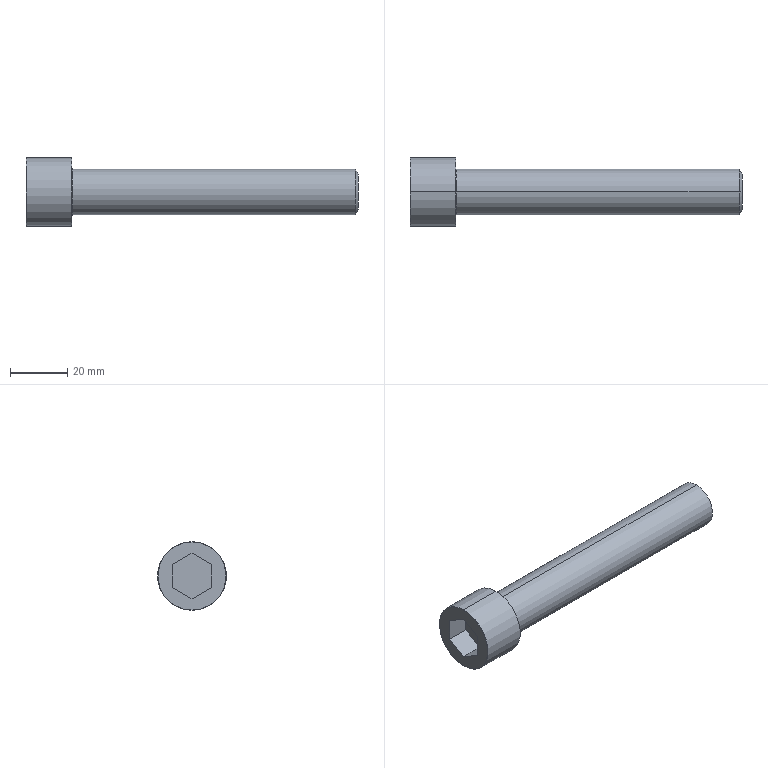Part | SolidWorks | features BlendCut 1, Cut 1, Fillet 1, LPattern 1, RevCut 1, Revolution 1 | 1 solid | 20 faces | box 116 x 24 x 24 mm | volume 25974 mm3 | plane 10 | torus 4 | cylinder 4 | cone 2 | commonest cylinder face diameters 16 x2 24 x2
STEP:
#1=CARTESIAN_POINT('',(0.,0.,11.9));
#2=VERTEX_POINT('',#1);
#3=CARTESIAN_POINT('',(0.,0.,-11.9));
#4=VERTEX_POINT('',#3);
#5=CARTESIAN_POINT('',(0.,0.,0.));
#6=DIRECTION('',(-1.,0.,0.));
#7=DIRECTION('',(0.,0.,-1.));
#8=AXIS2_PLACEMENT_3D('',#5,#6,#7);
#9=CIRCLE('',#8,11.9);
#10=EDGE_CURVE('',#2,#4,#9,.T.);
#11=ORIENTED_EDGE('',*,*,#10,.F.);
#12=CARTESIAN_POINT('',(0.1,0.,12.));
#13=VERTEX_POINT('',#12);
#14=CARTESIAN_POINT('',(0.1,0.,11.9));
#15=DIRECTION('',(0.,1.,0.));
#16=DIRECTION('',(0.,0.,1.));
#17=AXIS2_PLACEMENT_3D('',#14,#15,#16);
#18=CIRCLE('',#17,0.1);
#19=EDGE_CURVE('',#2,#13,#18,.T.);
#20=ORIENTED_EDGE('',*,*,#19,.T.);
#21=CARTESIAN_POINT('',(0.1,0.,-12.));
#22=VERTEX_POINT('',#21);
#23=CARTESIAN_POINT('',(0.1,0.,0.));
#24=DIRECTION('',(1.,0.,0.));
#25=DIRECTION('',(0.,0.,-1.));
#26=AXIS2_PLACEMENT_3D('',#23,#24,#25);
#27=CIRCLE('',#26,12.);
#28=EDGE_CURVE('',#22,#13,#27,.T.);
#29=ORIENTED_EDGE('',*,*,#28,.F.);
#30=CARTESIAN_POINT('',(0.1,0.,-11.9));
#31=DIRECTION('',(0.,-1.,0.));
#32=DIRECTION('',(0.,0.,-1.));
#33=AXIS2_PLACEMENT_3D('',#30,#31,#32);
#34=CIRCLE('',#33,0.1);
#35=EDGE_CURVE('',#4,#22,#34,.T.);
#36=ORIENTED_EDGE('',*,*,#35,.F.);
#37=EDGE_LOOP('',(#11,#20,#29,#36));
#38=FACE_OUTER_BOUND('',#37,.T.);
#39=CARTESIAN_POINT('',(0.1,0.,0.));
#40=DIRECTION('',(1.,0.,0.));
#41=DIRECTION('',(0.,0.,-1.));
#42=AXIS2_PLACEMENT_3D('',#39,#40,#41);
#43=TOROIDAL_SURFACE('',#42,11.9,0.1);
#44=ADVANCED_FACE('',(#38),#43,.T.);
#45=CARTESIAN_POINT('',(116.,0.,6.268));
#46=VERTEX_POINT('',#45);
#47=CARTESIAN_POINT('',(116.,0.,-6.268));
#48=VERTEX_POINT('',#47);
#49=CARTESIAN_POINT('',(116.,0.,0.));
#50=DIRECTION('',(-1.,0.,0.));
#51=DIRECTION('',(0.,0.,1.));
#52=AXIS2_PLACEMENT_3D('',#49,#50,#51);
#53=CIRCLE('',#52,6.268);
#54=EDGE_CURVE('',#46,#48,#53,.T.);
#55=ORIENTED_EDGE('',*,*,#54,.T.);
#56=CARTESIAN_POINT('',(115.,0.,-8.));
#57=VERTEX_POINT('',#56);
#58=CARTESIAN_POINT('',(115.,0.,-8.));
#59=DIRECTION('',(-0.5,0.,-0.866));
#60=VECTOR('',#59,1000.);
#61=LINE('',#58,#60);
#62=EDGE_CURVE('',#48,#57,#61,.T.);
#63=ORIENTED_EDGE('',*,*,#62,.T.);
#64=CARTESIAN_POINT('',(115.,0.,8.));
#65=VERTEX_POINT('',#64);
#66=CARTESIAN_POINT('',(115.,0.,0.));
#67=DIRECTION('',(-1.,0.,0.));
#68=DIRECTION('',(0.,0.,1.));
#69=AXIS2_PLACEMENT_3D('',#66,#67,#68);
#70=CIRCLE('',#69,8.);
#71=EDGE_CURVE('',#65,#57,#70,.T.);
#72=ORIENTED_EDGE('',*,*,#71,.F.);
#73=CARTESIAN_POINT('',(115.,0.,8.));
#74=DIRECTION('',(-0.5,0.,0.866));
#75=VECTOR('',#74,1000.);
#76=LINE('',#73,#75);
#77=EDGE_CURVE('',#46,#65,#76,.T.);
#78=ORIENTED_EDGE('',*,*,#77,.F.);
#79=EDGE_LOOP('',(#55,#63,#72,#78));
#80=FACE_OUTER_BOUND('',#79,.T.);
#81=CARTESIAN_POINT('',(115.,0.,0.));
#82=DIRECTION('',(-1.,0.,0.));
#83=DIRECTION('',(0.,0.,1.));
#84=AXIS2_PLACEMENT_3D('',#81,#82,#83);
#85=CONICAL_SURFACE('',#84,8.,1.047);
#86=ADVANCED_FACE('',(#80),#85,.T.);
#87=CARTESIAN_POINT('',(16.,0.,-8.2));
#88=VERTEX_POINT('',#87);
#89=CARTESIAN_POINT('',(16.,0.,8.2));
#90=VERTEX_POINT('',#89);
#91=CARTESIAN_POINT('',(16.,0.,0.));
#92=DIRECTION('',(-1.,0.,0.));
#93=DIRECTION('',(0.,0.,1.));
#94=AXIS2_PLACEMENT_3D('',#91,#92,#93);
#95=CIRCLE('',#94,8.2);
#96=EDGE_CURVE('',#88,#90,#95,.T.);
#97=ORIENTED_EDGE('',*,*,#96,.F.);
#98=CARTESIAN_POINT('',(16.2,0.,-8.));
#99=VERTEX_POINT('',#98);
#100=CARTESIAN_POINT('',(16.2,0.,-8.2));
#101=DIRECTION('',(0.,1.,0.));
#102=DIRECTION('',(0.,0.,1.));
#103=AXIS2_PLACEMENT_3D('',#100,#101,#102);
#104=CIRCLE('',#103,0.2);
#105=EDGE_CURVE('',#88,#99,#104,.T.);
#106=ORIENTED_EDGE('',*,*,#105,.T.);
#107=CARTESIAN_POINT('',(16.2,0.,8.));
#108=VERTEX_POINT('',#107);
#109=CARTESIAN_POINT('',(16.2,0.,0.));
#110=DIRECTION('',(-1.,0.,0.));
#111=DIRECTION('',(0.,0.,1.));
#112=AXIS2_PLACEMENT_3D('',#109,#110,#111);
#113=CIRCLE('',#112,8.);
#114=EDGE_CURVE('',#99,#108,#113,.T.);
#115=ORIENTED_EDGE('',*,*,#114,.T.);
#116=CARTESIAN_POINT('',(16.2,0.,8.2));
#117=DIRECTION('',(0.,-1.,0.));
#118=DIRECTION('',(0.,0.,-1.));
#119=AXIS2_PLACEMENT_3D('',#116,#117,#118);
#120=CIRCLE('',#119,0.2);
#121=EDGE_CURVE('',#90,#108,#120,.T.);
#122=ORIENTED_EDGE('',*,*,#121,.F.);
#123=EDGE_LOOP('',(#97,#106,#115,#122));
#124=FACE_OUTER_BOUND('',#123,.T.);
#125=CARTESIAN_POINT('',(16.2,0.,0.));
#126=DIRECTION('',(-1.,0.,0.));
#127=DIRECTION('',(0.,0.,1.));
#128=AXIS2_PLACEMENT_3D('',#125,#126,#127);
#129=TOROIDAL_SURFACE('',#128,8.2,0.2);
#130=ADVANCED_FACE('',(#124),#129,.F.);
#131=CARTESIAN_POINT('',(16.,0.,12.));
#132=VERTEX_POINT('',#131);
#133=CARTESIAN_POINT('',(16.,0.,-12.));
#134=VERTEX_POINT('',#133);
#135=CARTESIAN_POINT('',(16.,0.,0.));
#136=DIRECTION('',(-1.,0.,0.));
#137=DIRECTION('',(0.,0.,1.));
#138=AXIS2_PLACEMENT_3D('',#135,#136,#137);
#139=CIRCLE('',#138,12.);
#140=EDGE_CURVE('',#132,#134,#139,.T.);
#141=ORIENTED_EDGE('',*,*,#140,.T.);
#142=CARTESIAN_POINT('',(0.,0.,-12.));
#143=DIRECTION('',(-1.,0.,0.));
#144=VECTOR('',#143,1000.);
#145=LINE('',#142,#144);
#146=EDGE_CURVE('',#134,#22,#145,.T.);
#147=ORIENTED_EDGE('',*,*,#146,.T.);
#148=ORIENTED_EDGE('',*,*,#28,.T.);
#149=CARTESIAN_POINT('',(0.,0.,12.));
#150=DIRECTION('',(-1.,0.,0.));
#151=VECTOR('',#150,1000.);
#152=LINE('',#149,#151);
#153=EDGE_CURVE('',#132,#13,#152,.T.);
#154=ORIENTED_EDGE('',*,*,#153,.F.);
#155=EDGE_LOOP('',(#141,#147,#148,#154));
#156=FACE_OUTER_BOUND('',#155,.T.);
#157=CARTESIAN_POINT('',(0.,0.,0.));
#158=DIRECTION('',(-1.,0.,0.));
#159=DIRECTION('',(0.,0.,1.));
#160=AXIS2_PLACEMENT_3D('',#157,#158,#159);
#161=CYLINDRICAL_SURFACE('',#160,12.);
#162=ADVANCED_FACE('',(#156),#161,.T.);
#163=ORIENTED_EDGE('',*,*,#71,.T.);
#164=CARTESIAN_POINT('',(0.,0.,-8.));
#165=DIRECTION('',(-1.,0.,0.));
#166=VECTOR('',#165,1000.);
#167=LINE('',#164,#166);
#168=EDGE_CURVE('',#57,#99,#167,.T.);
#169=ORIENTED_EDGE('',*,*,#168,.T.);
#170=CARTESIAN_POINT('',(16.2,0.,0.));
#171=DIRECTION('',(-1.,0.,0.));
#172=DIRECTION('',(0.,0.,1.));
#173=AXIS2_PLACEMENT_3D('',#170,#171,#172);
#174=CIRCLE('',#173,8.);
#175=EDGE_CURVE('',#108,#99,#174,.T.);
#176=ORIENTED_EDGE('',*,*,#175,.F.);
#177=CARTESIAN_POINT('',(0.,0.,8.));
#178=DIRECTION('',(-1.,0.,0.));
#179=VECTOR('',#178,1000.);
#180=LINE('',#177,#179);
#181=EDGE_CURVE('',#65,#108,#180,.T.);
#182=ORIENTED_EDGE('',*,*,#181,.F.);
#183=EDGE_LOOP('',(#163,#169,#176,#182));
#184=FACE_OUTER_BOUND('',#183,.T.);
#185=CARTESIAN_POINT('',(0.,0.,0.));
#186=DIRECTION('',(-1.,0.,0.));
#187=DIRECTION('',(0.,0.,1.));
#188=AXIS2_PLACEMENT_3D('',#185,#186,#187);
#189=CYLINDRICAL_SURFACE('',#188,8.);
#190=ADVANCED_FACE('',(#184),#189,.T.);
#191=ORIENTED_EDGE('',*,*,#168,.F.);
#192=CARTESIAN_POINT('',(115.,0.,0.));
#193=DIRECTION('',(-1.,0.,0.));
#194=DIRECTION('',(0.,0.,1.));
#195=AXIS2_PLACEMENT_3D('',#192,#193,#194);
#196=CIRCLE('',#195,8.);
#197=EDGE_CURVE('',#57,#65,#196,.T.);
#198=ORIENTED_EDGE('',*,*,#197,.T.);
#199=ORIENTED_EDGE('',*,*,#181,.T.);
#200=ORIENTED_EDGE('',*,*,#114,.F.);
#201=EDGE_LOOP('',(#191,#198,#199,#200));
#202=FACE_OUTER_BOUND('',#201,.T.);
#203=CARTESIAN_POINT('',(0.,0.,0.));
#204=DIRECTION('',(-1.,0.,0.));
#205=DIRECTION('',(0.,0.,1.));
#206=AXIS2_PLACEMENT_3D('',#203,#204,#205);
#207=CYLINDRICAL_SURFACE('',#206,8.);
#208=ADVANCED_FACE('',(#202),#207,.T.);
#209=CARTESIAN_POINT('',(0.,0.,0.));
#210=DIRECTION('',(-1.,0.,0.));
#211=DIRECTION('',(0.,0.,-1.));
#212=AXIS2_PLACEMENT_3D('',#209,#210,#211);
#213=CIRCLE('',#212,11.9);
#214=EDGE_CURVE('',#4,#2,#213,.T.);
#215=ORIENTED_EDGE('',*,*,#214,.T.);
#216=ORIENTED_EDGE('',*,*,#10,.T.);
#217=EDGE_LOOP('',(#215,#216));
#218=FACE_OUTER_BOUND('',#217,.T.);
#219=CARTESIAN_POINT('',(0.,0.,8.));
#220=VERTEX_POINT('',#219);
#221=CARTESIAN_POINT('',(0.,6.928,4.));
#222=VERTEX_POINT('',#221);
#223=CARTESIAN_POINT('',(0.,0.,8.));
#224=DIRECTION('',(0.,0.866,-0.5));
#225=VECTOR('',#224,1000.);
#226=LINE('',#223,#225);
#227=EDGE_CURVE('',#220,#222,#226,.T.);
#228=ORIENTED_EDGE('',*,*,#227,.F.);
#229=CARTESIAN_POINT('',(0.,-6.928,4.));
#230=VERTEX_POINT('',#229);
#231=CARTESIAN_POINT('',(0.,-6.928,4.));
#232=DIRECTION('',(0.,0.866,0.5));
#233=VECTOR('',#232,1000.);
#234=LINE('',#231,#233);
#235=EDGE_CURVE('',#230,#220,#234,.T.);
#236=ORIENTED_EDGE('',*,*,#235,.F.);
#237=CARTESIAN_POINT('',(0.,-6.928,-4.));
#238=VERTEX_POINT('',#237);
#239=CARTESIAN_POINT('',(0.,-6.928,-4.));
#240=DIRECTION('',(0.,0.,1.));
#241=VECTOR('',#240,1000.);
#242=LINE('',#239,#241);
#243=EDGE_CURVE('',#238,#230,#242,.T.);
#244=ORIENTED_EDGE('',*,*,#243,.F.);
#245=CARTESIAN_POINT('',(0.,0.,-8.));
#246=VERTEX_POINT('',#245);
#247=CARTESIAN_POINT('',(0.,0.,-8.));
#248=DIRECTION('',(0.,-0.866,0.5));
#249=VECTOR('',#248,1000.);
#250=LINE('',#247,#249);
#251=EDGE_CURVE('',#246,#238,#250,.T.);
#252=ORIENTED_EDGE('',*,*,#251,.F.);
#253=CARTESIAN_POINT('',(0.,6.928,-4.));
#254=VERTEX_POINT('',#253);
#255=CARTESIAN_POINT('',(0.,6.928,-4.));
#256=DIRECTION('',(0.,-0.866,-0.5));
#257=VECTOR('',#256,1000.);
#258=LINE('',#255,#257);
#259=EDGE_CURVE('',#254,#246,#258,.T.);
#260=ORIENTED_EDGE('',*,*,#259,.F.);
#261=CARTESIAN_POINT('',(0.,6.928,4.));
#262=DIRECTION('',(0.,0.,-1.));
#263=VECTOR('',#262,1000.);
#264=LINE('',#261,#263);
#265=EDGE_CURVE('',#222,#254,#264,.T.);
#266=ORIENTED_EDGE('',*,*,#265,.F.);
#267=EDGE_LOOP('',(#228,#236,#244,#252,#260,#266));
#268=FACE_BOUND('',#267,.T.);
#269=CARTESIAN_POINT('',(0.,0.,0.));
#270=DIRECTION('',(1.,0.,0.));
#271=DIRECTION('',(0.,0.,-1.));
#272=AXIS2_PLACEMENT_3D('',#269,#270,#271);
#273=PLANE('',#272);
#274=ADVANCED_FACE('',(#218,#268),#273,.F.);
#275=ORIENTED_EDGE('',*,*,#146,.F.);
#276=CARTESIAN_POINT('',(16.,0.,0.));
#277=DIRECTION('',(-1.,0.,0.));
#278=DIRECTION('',(0.,0.,1.));
#279=AXIS2_PLACEMENT_3D('',#276,#277,#278);
#280=CIRCLE('',#279,12.);
#281=EDGE_CURVE('',#134,#132,#280,.T.);
#282=ORIENTED_EDGE('',*,*,#281,.T.);
#283=ORIENTED_EDGE('',*,*,#153,.T.);
#284=CARTESIAN_POINT('',(0.1,0.,0.));
#285=DIRECTION('',(1.,0.,0.));
#286=DIRECTION('',(0.,0.,-1.));
#287=AXIS2_PLACEMENT_3D('',#284,#285,#286);
#288=CIRCLE('',#287,12.);
#289=EDGE_CURVE('',#13,#22,#288,.T.);
#290=ORIENTED_EDGE('',*,*,#289,.T.);
#291=EDGE_LOOP('',(#275,#282,#283,#290));
#292=FACE_OUTER_BOUND('',#291,.T.);
#293=CARTESIAN_POINT('',(0.,0.,0.));
#294=DIRECTION('',(-1.,0.,0.));
#295=DIRECTION('',(0.,0.,1.));
#296=AXIS2_PLACEMENT_3D('',#293,#294,#295);
#297=CYLINDRICAL_SURFACE('',#296,12.);
#298=ADVANCED_FACE('',(#292),#297,.T.);
#299=ORIENTED_EDGE('',*,*,#140,.F.);
#300=ORIENTED_EDGE('',*,*,#281,.F.);
#301=EDGE_LOOP('',(#299,#300));
#302=FACE_OUTER_BOUND('',#301,.T.);
#303=CARTESIAN_POINT('',(16.,0.,0.));
#304=DIRECTION('',(-1.,0.,0.));
#305=DIRECTION('',(0.,0.,1.));
#306=AXIS2_PLACEMENT_3D('',#303,#304,#305);
#307=CIRCLE('',#306,8.2);
#308=EDGE_CURVE('',#90,#88,#307,.T.);
#309=ORIENTED_EDGE('',*,*,#308,.T.);
#310=ORIENTED_EDGE('',*,*,#96,.T.);
#311=EDGE_LOOP('',(#309,#310));
#312=FACE_BOUND('',#311,.T.);
#313=CARTESIAN_POINT('',(16.,12.,0.));
#314=DIRECTION('',(-1.,0.,0.));
#315=DIRECTION('',(0.,0.,1.));
#316=AXIS2_PLACEMENT_3D('',#313,#314,#315);
#317=PLANE('',#316);
#318=ADVANCED_FACE('',(#302,#312),#317,.F.);
#319=ORIENTED_EDGE('',*,*,#105,.F.);
#320=ORIENTED_EDGE('',*,*,#308,.F.);
#321=ORIENTED_EDGE('',*,*,#121,.T.);
#322=ORIENTED_EDGE('',*,*,#175,.T.);
#323=EDGE_LOOP('',(#319,#320,#321,#322));
#324=FACE_OUTER_BOUND('',#323,.T.);
#325=CARTESIAN_POINT('',(16.2,0.,0.));
#326=DIRECTION('',(-1.,0.,0.));
#327=DIRECTION('',(0.,0.,1.));
#328=AXIS2_PLACEMENT_3D('',#325,#326,#327);
#329=TOROIDAL_SURFACE('',#328,8.2,0.2);
#330=ADVANCED_FACE('',(#324),#329,.F.);
#331=ORIENTED_EDGE('',*,*,#235,.T.);
#332=CARTESIAN_POINT('',(8.,0.,8.));
#333=VERTEX_POINT('',#332);
#334=CARTESIAN_POINT('',(8.,0.,8.));
#335=DIRECTION('',(-1.,0.,0.));
#336=VECTOR('',#335,1000.);
#337=LINE('',#334,#336);
#338=EDGE_CURVE('',#333,#220,#337,.T.);
#339=ORIENTED_EDGE('',*,*,#338,.F.);
#340=CARTESIAN_POINT('',(8.,-6.928,4.));
#341=VERTEX_POINT('',#340);
#342=CARTESIAN_POINT('',(8.,-6.928,4.));
#343=DIRECTION('',(0.,0.866,0.5));
#344=VECTOR('',#343,1000.);
#345=LINE('',#342,#344);
#346=EDGE_CURVE('',#341,#333,#345,.T.);
#347=ORIENTED_EDGE('',*,*,#346,.F.);
#348=CARTESIAN_POINT('',(8.,-6.928,4.));
#349=DIRECTION('',(-1.,0.,0.));
#350=VECTOR('',#349,1000.);
#351=LINE('',#348,#350);
#352=EDGE_CURVE('',#341,#230,#351,.T.);
#353=ORIENTED_EDGE('',*,*,#352,.T.);
#354=EDGE_LOOP('',(#331,#339,#347,#353));
#355=FACE_OUTER_BOUND('',#354,.T.);
#356=CARTESIAN_POINT('',(8.,-6.928,4.));
#357=DIRECTION('',(0.,-0.5,0.866));
#358=DIRECTION('',(0.,-0.866,-0.5));
#359=AXIS2_PLACEMENT_3D('',#356,#357,#358);
#360=PLANE('',#359);
#361=ADVANCED_FACE('',(#355),#360,.F.);
#362=ORIENTED_EDGE('',*,*,#243,.T.);
#363=ORIENTED_EDGE('',*,*,#352,.F.);
#364=CARTESIAN_POINT('',(8.,-6.928,-4.));
#365=VERTEX_POINT('',#364);
#366=CARTESIAN_POINT('',(8.,-6.928,-4.));
#367=DIRECTION('',(0.,0.,1.));
#368=VECTOR('',#367,1000.);
#369=LINE('',#366,#368);
#370=EDGE_CURVE('',#365,#341,#369,.T.);
#371=ORIENTED_EDGE('',*,*,#370,.F.);
#372=CARTESIAN_POINT('',(8.,-6.928,-4.));
#373=DIRECTION('',(-1.,0.,0.));
#374=VECTOR('',#373,1000.);
#375=LINE('',#372,#374);
#376=EDGE_CURVE('',#365,#238,#375,.T.);
#377=ORIENTED_EDGE('',*,*,#376,.T.);
#378=EDGE_LOOP('',(#362,#363,#371,#377));
#379=FACE_OUTER_BOUND('',#378,.T.);
#380=CARTESIAN_POINT('',(8.,-6.928,-4.));
#381=DIRECTION('',(0.,-1.,0.));
#382=DIRECTION('',(0.,0.,-1.));
#383=AXIS2_PLACEMENT_3D('',#380,#381,#382);
#384=PLANE('',#383);
#385=ADVANCED_FACE('',(#379),#384,.F.);
#386=ORIENTED_EDGE('',*,*,#251,.T.);
#387=ORIENTED_EDGE('',*,*,#376,.F.);
#388=CARTESIAN_POINT('',(8.,0.,-8.));
#389=VERTEX_POINT('',#388);
#390=CARTESIAN_POINT('',(8.,0.,-8.));
#391=DIRECTION('',(0.,-0.866,0.5));
#392=VECTOR('',#391,1000.);
#393=LINE('',#390,#392);
#394=EDGE_CURVE('',#389,#365,#393,.T.);
#395=ORIENTED_EDGE('',*,*,#394,.F.);
#396=CARTESIAN_POINT('',(8.,0.,-8.));
#397=DIRECTION('',(-1.,0.,0.));
#398=VECTOR('',#397,1000.);
#399=LINE('',#396,#398);
#400=EDGE_CURVE('',#389,#246,#399,.T.);
#401=ORIENTED_EDGE('',*,*,#400,.T.);
#402=EDGE_LOOP('',(#386,#387,#395,#401));
#403=FACE_OUTER_BOUND('',#402,.T.);
#404=CARTESIAN_POINT('',(8.,0.,-8.));
#405=DIRECTION('',(0.,-0.5,-0.866));
#406=DIRECTION('',(0.,0.866,-0.5));
#407=AXIS2_PLACEMENT_3D('',#404,#405,#406);
#408=PLANE('',#407);
#409=ADVANCED_FACE('',(#403),#408,.F.);
#410=ORIENTED_EDGE('',*,*,#259,.T.);
#411=ORIENTED_EDGE('',*,*,#400,.F.);
#412=CARTESIAN_POINT('',(8.,6.928,-4.));
#413=VERTEX_POINT('',#412);
#414=CARTESIAN_POINT('',(8.,6.928,-4.));
#415=DIRECTION('',(0.,-0.866,-0.5));
#416=VECTOR('',#415,1000.);
#417=LINE('',#414,#416);
#418=EDGE_CURVE('',#413,#389,#417,.T.);
#419=ORIENTED_EDGE('',*,*,#418,.F.);
#420=CARTESIAN_POINT('',(8.,6.928,-4.));
#421=DIRECTION('',(-1.,0.,0.));
#422=VECTOR('',#421,1000.);
#423=LINE('',#420,#422);
#424=EDGE_CURVE('',#413,#254,#423,.T.);
#425=ORIENTED_EDGE('',*,*,#424,.T.);
#426=EDGE_LOOP('',(#410,#411,#419,#425));
#427=FACE_OUTER_BOUND('',#426,.T.);
#428=CARTESIAN_POINT('',(8.,6.928,-4.));
#429=DIRECTION('',(0.,0.5,-0.866));
#430=DIRECTION('',(0.,0.866,0.5));
#431=AXIS2_PLACEMENT_3D('',#428,#429,#430);
#432=PLANE('',#431);
#433=ADVANCED_FACE('',(#427),#432,.F.);
#434=ORIENTED_EDGE('',*,*,#265,.T.);
#435=ORIENTED_EDGE('',*,*,#424,.F.);
#436=CARTESIAN_POINT('',(8.,6.928,4.));
#437=VERTEX_POINT('',#436);
#438=CARTESIAN_POINT('',(8.,6.928,4.));
#439=DIRECTION('',(0.,0.,-1.));
#440=VECTOR('',#439,1000.);
#441=LINE('',#438,#440);
#442=EDGE_CURVE('',#437,#413,#441,.T.);
#443=ORIENTED_EDGE('',*,*,#442,.F.);
#444=CARTESIAN_POINT('',(8.,6.928,4.));
#445=DIRECTION('',(-1.,0.,0.));
#446=VECTOR('',#445,1000.);
#447=LINE('',#444,#446);
#448=EDGE_CURVE('',#437,#222,#447,.T.);
#449=ORIENTED_EDGE('',*,*,#448,.T.);
#450=EDGE_LOOP('',(#434,#435,#443,#449));
#451=FACE_OUTER_BOUND('',#450,.T.);
#452=CARTESIAN_POINT('',(8.,6.928,4.));
#453=DIRECTION('',(0.,1.,0.));
#454=DIRECTION('',(0.,0.,1.));
#455=AXIS2_PLACEMENT_3D('',#452,#453,#454);
#456=PLANE('',#455);
#457=ADVANCED_FACE('',(#451),#456,.F.);
#458=ORIENTED_EDGE('',*,*,#227,.T.);
#459=ORIENTED_EDGE('',*,*,#448,.F.);
#460=CARTESIAN_POINT('',(8.,0.,8.));
#461=DIRECTION('',(0.,0.866,-0.5));
#462=VECTOR('',#461,1000.);
#463=LINE('',#460,#462);
#464=EDGE_CURVE('',#333,#437,#463,.T.);
#465=ORIENTED_EDGE('',*,*,#464,.F.);
#466=ORIENTED_EDGE('',*,*,#338,.T.);
#467=EDGE_LOOP('',(#458,#459,#465,#466));
#468=FACE_OUTER_BOUND('',#467,.T.);
#469=CARTESIAN_POINT('',(8.,0.,8.));
#470=DIRECTION('',(0.,0.5,0.866));
#471=DIRECTION('',(0.,-0.866,0.5));
#472=AXIS2_PLACEMENT_3D('',#469,#470,#471);
#473=PLANE('',#472);
#474=ADVANCED_FACE('',(#468),#473,.F.);
#475=ORIENTED_EDGE('',*,*,#346,.T.);
#476=ORIENTED_EDGE('',*,*,#464,.T.);
#477=ORIENTED_EDGE('',*,*,#442,.T.);
#478=ORIENTED_EDGE('',*,*,#418,.T.);
#479=ORIENTED_EDGE('',*,*,#394,.T.);
#480=ORIENTED_EDGE('',*,*,#370,.T.);
#481=EDGE_LOOP('',(#475,#476,#477,#478,#479,#480));
#482=FACE_OUTER_BOUND('',#481,.T.);
#483=CARTESIAN_POINT('',(8.,-6.928,4.));
#484=DIRECTION('',(1.,0.,0.));
#485=DIRECTION('',(0.,0.,-1.));
#486=AXIS2_PLACEMENT_3D('',#483,#484,#485);
#487=PLANE('',#486);
#488=ADVANCED_FACE('',(#482),#487,.F.);
#489=ORIENTED_EDGE('',*,*,#62,.F.);
#490=CARTESIAN_POINT('',(116.,0.,0.));
#491=DIRECTION('',(-1.,0.,0.));
#492=DIRECTION('',(0.,0.,1.));
#493=AXIS2_PLACEMENT_3D('',#490,#491,#492);
#494=CIRCLE('',#493,6.268);
#495=EDGE_CURVE('',#48,#46,#494,.T.);
#496=ORIENTED_EDGE('',*,*,#495,.T.);
#497=ORIENTED_EDGE('',*,*,#77,.T.);
#498=ORIENTED_EDGE('',*,*,#197,.F.);
#499=EDGE_LOOP('',(#489,#496,#497,#498));
#500=FACE_OUTER_BOUND('',#499,.T.);
#501=CARTESIAN_POINT('',(115.,0.,0.));
#502=DIRECTION('',(-1.,0.,0.));
#503=DIRECTION('',(0.,0.,1.));
#504=AXIS2_PLACEMENT_3D('',#501,#502,#503);
#505=CONICAL_SURFACE('',#504,8.,1.047);
#506=ADVANCED_FACE('',(#500),#505,.T.);
#507=ORIENTED_EDGE('',*,*,#54,.F.);
#508=ORIENTED_EDGE('',*,*,#495,.F.);
#509=EDGE_LOOP('',(#507,#508));
#510=FACE_OUTER_BOUND('',#509,.T.);
#511=CARTESIAN_POINT('',(116.,8.,0.));
#512=DIRECTION('',(-1.,0.,0.));
#513=DIRECTION('',(0.,0.,1.));
#514=AXIS2_PLACEMENT_3D('',#511,#512,#513);
#515=PLANE('',#514);
#516=ADVANCED_FACE('',(#510),#515,.F.);
#517=ORIENTED_EDGE('',*,*,#19,.F.);
#518=ORIENTED_EDGE('',*,*,#214,.F.);
#519=ORIENTED_EDGE('',*,*,#35,.T.);
#520=ORIENTED_EDGE('',*,*,#289,.F.);
#521=EDGE_LOOP('',(#517,#518,#519,#520));
#522=FACE_OUTER_BOUND('',#521,.T.);
#523=CARTESIAN_POINT('',(0.1,0.,0.));
#524=DIRECTION('',(1.,0.,0.));
#525=DIRECTION('',(0.,0.,-1.));
#526=AXIS2_PLACEMENT_3D('',#523,#524,#525);
#527=TOROIDAL_SURFACE('',#526,11.9,0.1);
#528=ADVANCED_FACE('',(#522),#527,.T.);
#529=CLOSED_SHELL('',(#44,#86,#130,#162,#190,#208,#274,#298,#318,#330,#361,#385,#409,#433,#457,#474,#488,#506,#516,#528));
#530=MANIFOLD_SOLID_BREP('',#529);
#531=CARTESIAN_POINT('',(0.,0.,0.));
#532=DIRECTION('',(0.,0.,1.));
#533=DIRECTION('',(1.,0.,0.));
#534=AXIS2_PLACEMENT_3D('',#531,#532,#533);
#535=(LENGTH_UNIT()NAMED_UNIT(*)SI_UNIT(.MILLI.,.METRE.));
#536=UNCERTAINTY_MEASURE_WITH_UNIT(LENGTH_MEASURE(0.00001),#535,'','');
#537=(NAMED_UNIT(*)PLANE_ANGLE_UNIT()SI_UNIT($,.RADIAN.));
#538=(NAMED_UNIT(*)SI_UNIT($,.STERADIAN.)SOLID_ANGLE_UNIT());
#539=(GEOMETRIC_REPRESENTATION_CONTEXT(3)GLOBAL_UNCERTAINTY_ASSIGNED_CONTEXT((#536))GLOBAL_UNIT_ASSIGNED_CONTEXT((#535,#537,#538))REPRESENTATION_CONTEXT('',''));
#540=ADVANCED_BREP_SHAPE_REPRESENTATION('',(#530,#534),#539);